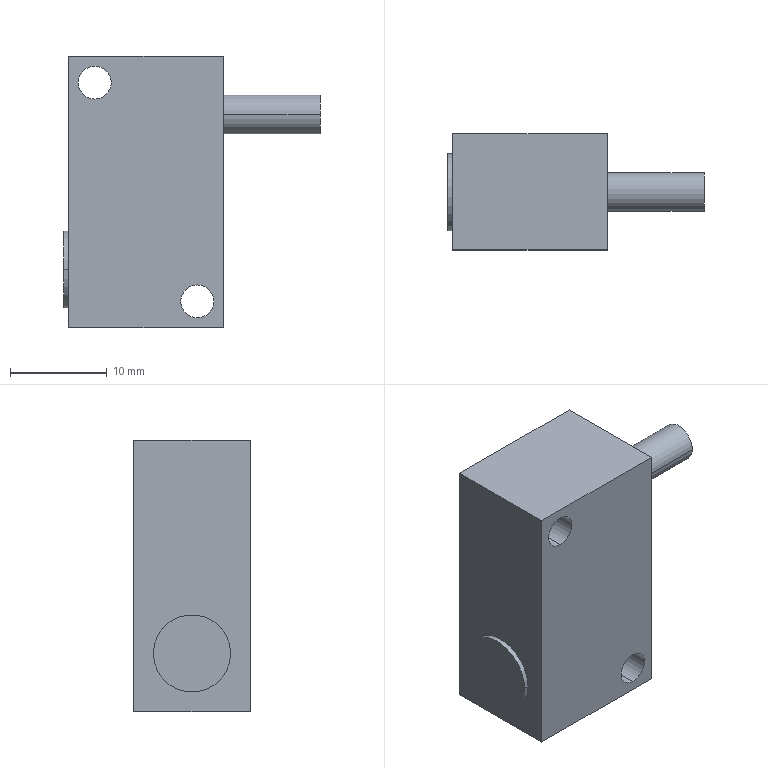Part | STEP file | Square proximity switch | 1 solid | 16 faces | box 26.5 x 12 x 28 mm | volume 5309 mm3 | cylinder 8 | plane 8 | commonest cylinder face diameters 3.4 x4 4 x2 8 x2
STEP:
#1=CARTESIAN_POINT('',(0.,0.,0.));
#2=DIRECTION('',(0.,0.,1.));
#3=DIRECTION('',(1.,0.,0.));
#4=AXIS2_PLACEMENT_3D('',#1,#2,#3);
#5=CARTESIAN_POINT('',(-5.3,6.,23.6));
#6=VERTEX_POINT('',#5);
#7=CARTESIAN_POINT('',(-5.3,-6.,23.6));
#8=VERTEX_POINT('',#7);
#9=CARTESIAN_POINT('',(-5.3,-6.,23.6));
#10=DIRECTION('',(0.,-1.,0.));
#11=VECTOR('',#10,1.);
#12=LINE('',#9,#11);
#13=CARTESIAN_POINT('',(-5.3,-6.,25.3));
#14=DIRECTION('',(0.,-1.,0.));
#15=DIRECTION('',(0.,0.,-1.));
#16=AXIS2_PLACEMENT_3D('',#13,#14,#15);
#17=CYLINDRICAL_SURFACE('',#16,1.7);
#18=CARTESIAN_POINT('',(6.283,0.));
#19=DIRECTION('',(0.,1.));
#20=VECTOR('',#19,1.);
#21=LINE('',#18,#20);
#22=(GEOMETRIC_REPRESENTATION_CONTEXT(2)PARAMETRIC_REPRESENTATION_CONTEXT()REPRESENTATION_CONTEXT('',''));
#23=DEFINITIONAL_REPRESENTATION('',(#21),#22);
#24=PCURVE('',#17,#23);
#25=CARTESIAN_POINT('',(-5.3,-6.,25.3));
#26=DIRECTION('',(0.,-1.,0.));
#27=DIRECTION('',(0.,0.,-1.));
#28=AXIS2_PLACEMENT_3D('',#25,#26,#27);
#29=CYLINDRICAL_SURFACE('',#28,1.7);
#30=CARTESIAN_POINT('',(0.,0.));
#31=DIRECTION('',(0.,1.));
#32=VECTOR('',#31,1.);
#33=LINE('',#30,#32);
#34=(GEOMETRIC_REPRESENTATION_CONTEXT(2)PARAMETRIC_REPRESENTATION_CONTEXT()REPRESENTATION_CONTEXT('',''));
#35=DEFINITIONAL_REPRESENTATION('',(#33),#34);
#36=PCURVE('',#29,#35);
#37=SURFACE_CURVE('',#12,(#24,#36),.PCURVE_S1.);
#38=EDGE_CURVE('',#6,#8,#37,.T.);
#39=ORIENTED_EDGE('',*,*,#38,.T.);
#40=CARTESIAN_POINT('',(-5.3,-6.,27.));
#41=VERTEX_POINT('',#40);
#42=CARTESIAN_POINT('',(-5.3,-6.,25.3));
#43=DIRECTION('',(0.,-1.,0.));
#44=DIRECTION('',(0.,0.,-1.));
#45=AXIS2_PLACEMENT_3D('',#42,#43,#44);
#46=CIRCLE('',#45,1.7);
#47=CARTESIAN_POINT('',(0.,0.));
#48=DIRECTION('',(1.,0.));
#49=VECTOR('',#48,1.);
#50=LINE('',#47,#49);
#51=(GEOMETRIC_REPRESENTATION_CONTEXT(2)PARAMETRIC_REPRESENTATION_CONTEXT()REPRESENTATION_CONTEXT('',''));
#52=DEFINITIONAL_REPRESENTATION('',(#50),#51);
#53=PCURVE('',#17,#52);
#54=CARTESIAN_POINT('',(-8.,-6.,28.));
#55=DIRECTION('',(0.,1.,0.));
#56=DIRECTION('',(0.,0.,1.));
#57=AXIS2_PLACEMENT_3D('',#54,#55,#56);
#58=PLANE('',#57);
#59=CARTESIAN_POINT('',(-4.4,2.7));
#60=CARTESIAN_POINT('',(-4.4,5.644));
#61=CARTESIAN_POINT('',(-1.85,4.172));
#62=CARTESIAN_POINT('',(0.7,2.7));
#63=CARTESIAN_POINT('',(-1.85,1.228));
#64=CARTESIAN_POINT('',(-4.4,-0.2445));
#65=CARTESIAN_POINT('',(-4.4,2.7));
#66=(BOUNDED_CURVE()B_SPLINE_CURVE(2,(#59,#60,#61,#62,#63,#64,#65),.UNSPECIFIED.,.T.,.F.)B_SPLINE_CURVE_WITH_KNOTS((1,2,2,2,2,1),(-2.094,0.,2.094,4.189,6.283,8.378),.UNSPECIFIED.)CURVE()GEOMETRIC_REPRESENTATION_ITEM()RATIONAL_B_SPLINE_CURVE((1.,0.5,1.,0.5,1.,0.5,1.))REPRESENTATION_ITEM(''));
#67=(GEOMETRIC_REPRESENTATION_CONTEXT(2)PARAMETRIC_REPRESENTATION_CONTEXT()REPRESENTATION_CONTEXT('',''));
#68=DEFINITIONAL_REPRESENTATION('',(#66),#67);
#69=PCURVE('',#58,#68);
#70=SURFACE_CURVE('',#46,(#53,#69),.PCURVE_S1.);
#71=EDGE_CURVE('',#41,#8,#70,.T.);
#72=ORIENTED_EDGE('',*,*,#71,.F.);
#73=CARTESIAN_POINT('',(-5.3,6.,27.));
#74=VERTEX_POINT('',#73);
#75=CARTESIAN_POINT('',(-5.3,-6.,27.));
#76=DIRECTION('',(0.,-1.,0.));
#77=VECTOR('',#76,1.);
#78=LINE('',#75,#77);
#79=CARTESIAN_POINT('',(3.142,0.));
#80=DIRECTION('',(0.,1.));
#81=VECTOR('',#80,1.);
#82=LINE('',#79,#81);
#83=(GEOMETRIC_REPRESENTATION_CONTEXT(2)PARAMETRIC_REPRESENTATION_CONTEXT()REPRESENTATION_CONTEXT('',''));
#84=DEFINITIONAL_REPRESENTATION('',(#82),#83);
#85=PCURVE('',#17,#84);
#86=CARTESIAN_POINT('',(3.142,0.));
#87=DIRECTION('',(0.,1.));
#88=VECTOR('',#87,1.);
#89=LINE('',#86,#88);
#90=(GEOMETRIC_REPRESENTATION_CONTEXT(2)PARAMETRIC_REPRESENTATION_CONTEXT()REPRESENTATION_CONTEXT('',''));
#91=DEFINITIONAL_REPRESENTATION('',(#89),#90);
#92=PCURVE('',#29,#91);
#93=SURFACE_CURVE('',#78,(#85,#92),.PCURVE_S1.);
#94=EDGE_CURVE('',#74,#41,#93,.T.);
#95=ORIENTED_EDGE('',*,*,#94,.F.);
#96=CARTESIAN_POINT('',(-5.3,6.,25.3));
#97=DIRECTION('',(0.,-1.,0.));
#98=DIRECTION('',(0.,0.,-1.));
#99=AXIS2_PLACEMENT_3D('',#96,#97,#98);
#100=CIRCLE('',#99,1.7);
#101=CARTESIAN_POINT('',(0.,-12.));
#102=DIRECTION('',(1.,0.));
#103=VECTOR('',#102,1.);
#104=LINE('',#101,#103);
#105=(GEOMETRIC_REPRESENTATION_CONTEXT(2)PARAMETRIC_REPRESENTATION_CONTEXT()REPRESENTATION_CONTEXT('',''));
#106=DEFINITIONAL_REPRESENTATION('',(#104),#105);
#107=PCURVE('',#17,#106);
#108=CARTESIAN_POINT('',(-8.,6.,28.));
#109=DIRECTION('',(0.,-1.,0.));
#110=DIRECTION('',(0.,0.,-1.));
#111=AXIS2_PLACEMENT_3D('',#108,#109,#110);
#112=PLANE('',#111);
#113=CARTESIAN_POINT('',(2.7,2.7));
#114=DIRECTION('',(1.,0.));
#115=AXIS2_PLACEMENT_2D('',#113,#114);
#116=CIRCLE('',#115,1.7);
#117=(GEOMETRIC_REPRESENTATION_CONTEXT(2)PARAMETRIC_REPRESENTATION_CONTEXT()REPRESENTATION_CONTEXT('',''));
#118=DEFINITIONAL_REPRESENTATION('',(#116),#117);
#119=PCURVE('',#112,#118);
#120=SURFACE_CURVE('',#100,(#107,#119),.PCURVE_S1.);
#121=EDGE_CURVE('',#74,#6,#120,.T.);
#122=ORIENTED_EDGE('',*,*,#121,.T.);
#123=EDGE_LOOP('',(#39,#72,#95,#122));
#124=FACE_BOUND('',#123,.F.);
#125=ADVANCED_FACE('',(#124),#17,.F.);
#126=CARTESIAN_POINT('',(5.3,6.,1.));
#127=VERTEX_POINT('',#126);
#128=CARTESIAN_POINT('',(5.3,-6.,1.));
#129=VERTEX_POINT('',#128);
#130=CARTESIAN_POINT('',(5.3,-6.,1.));
#131=DIRECTION('',(0.,-1.,0.));
#132=VECTOR('',#131,1.);
#133=LINE('',#130,#132);
#134=CARTESIAN_POINT('',(5.3,-6.,2.7));
#135=DIRECTION('',(0.,-1.,0.));
#136=DIRECTION('',(0.,0.,-1.));
#137=AXIS2_PLACEMENT_3D('',#134,#135,#136);
#138=CYLINDRICAL_SURFACE('',#137,1.7);
#139=CARTESIAN_POINT('',(6.283,0.));
#140=DIRECTION('',(0.,1.));
#141=VECTOR('',#140,1.);
#142=LINE('',#139,#141);
#143=(GEOMETRIC_REPRESENTATION_CONTEXT(2)PARAMETRIC_REPRESENTATION_CONTEXT()REPRESENTATION_CONTEXT('',''));
#144=DEFINITIONAL_REPRESENTATION('',(#142),#143);
#145=PCURVE('',#138,#144);
#146=CARTESIAN_POINT('',(5.3,-6.,2.7));
#147=DIRECTION('',(0.,-1.,0.));
#148=DIRECTION('',(0.,0.,-1.));
#149=AXIS2_PLACEMENT_3D('',#146,#147,#148);
#150=CYLINDRICAL_SURFACE('',#149,1.7);
#151=CARTESIAN_POINT('',(0.,0.));
#152=DIRECTION('',(0.,1.));
#153=VECTOR('',#152,1.);
#154=LINE('',#151,#153);
#155=(GEOMETRIC_REPRESENTATION_CONTEXT(2)PARAMETRIC_REPRESENTATION_CONTEXT()REPRESENTATION_CONTEXT('',''));
#156=DEFINITIONAL_REPRESENTATION('',(#154),#155);
#157=PCURVE('',#150,#156);
#158=SURFACE_CURVE('',#133,(#145,#157),.PCURVE_S1.);
#159=EDGE_CURVE('',#127,#129,#158,.T.);
#160=ORIENTED_EDGE('',*,*,#159,.T.);
#161=CARTESIAN_POINT('',(5.3,-6.,4.4));
#162=VERTEX_POINT('',#161);
#163=CARTESIAN_POINT('',(5.3,-6.,2.7));
#164=DIRECTION('',(0.,-1.,0.));
#165=DIRECTION('',(0.,0.,-1.));
#166=AXIS2_PLACEMENT_3D('',#163,#164,#165);
#167=CIRCLE('',#166,1.7);
#168=CARTESIAN_POINT('',(0.,0.));
#169=DIRECTION('',(1.,0.));
#170=VECTOR('',#169,1.);
#171=LINE('',#168,#170);
#172=(GEOMETRIC_REPRESENTATION_CONTEXT(2)PARAMETRIC_REPRESENTATION_CONTEXT()REPRESENTATION_CONTEXT('',''));
#173=DEFINITIONAL_REPRESENTATION('',(#171),#172);
#174=PCURVE('',#138,#173);
#175=CARTESIAN_POINT('',(-27.,13.3));
#176=CARTESIAN_POINT('',(-27.,16.244));
#177=CARTESIAN_POINT('',(-24.45,14.772));
#178=CARTESIAN_POINT('',(-21.9,13.3));
#179=CARTESIAN_POINT('',(-24.45,11.828));
#180=CARTESIAN_POINT('',(-27.,10.356));
#181=CARTESIAN_POINT('',(-27.,13.3));
#182=(BOUNDED_CURVE()B_SPLINE_CURVE(2,(#175,#176,#177,#178,#179,#180,#181),.UNSPECIFIED.,.T.,.F.)B_SPLINE_CURVE_WITH_KNOTS((1,2,2,2,2,1),(-2.094,0.,2.094,4.189,6.283,8.378),.UNSPECIFIED.)CURVE()GEOMETRIC_REPRESENTATION_ITEM()RATIONAL_B_SPLINE_CURVE((1.,0.5,1.,0.5,1.,0.5,1.))REPRESENTATION_ITEM(''));
#183=(GEOMETRIC_REPRESENTATION_CONTEXT(2)PARAMETRIC_REPRESENTATION_CONTEXT()REPRESENTATION_CONTEXT('',''));
#184=DEFINITIONAL_REPRESENTATION('',(#182),#183);
#185=PCURVE('',#58,#184);
#186=SURFACE_CURVE('',#167,(#174,#185),.PCURVE_S1.);
#187=EDGE_CURVE('',#162,#129,#186,.T.);
#188=ORIENTED_EDGE('',*,*,#187,.F.);
#189=CARTESIAN_POINT('',(5.3,6.,4.4));
#190=VERTEX_POINT('',#189);
#191=CARTESIAN_POINT('',(5.3,-6.,4.4));
#192=DIRECTION('',(0.,-1.,0.));
#193=VECTOR('',#192,1.);
#194=LINE('',#191,#193);
#195=CARTESIAN_POINT('',(3.142,0.));
#196=DIRECTION('',(0.,1.));
#197=VECTOR('',#196,1.);
#198=LINE('',#195,#197);
#199=(GEOMETRIC_REPRESENTATION_CONTEXT(2)PARAMETRIC_REPRESENTATION_CONTEXT()REPRESENTATION_CONTEXT('',''));
#200=DEFINITIONAL_REPRESENTATION('',(#198),#199);
#201=PCURVE('',#138,#200);
#202=CARTESIAN_POINT('',(3.142,0.));
#203=DIRECTION('',(0.,1.));
#204=VECTOR('',#203,1.);
#205=LINE('',#202,#204);
#206=(GEOMETRIC_REPRESENTATION_CONTEXT(2)PARAMETRIC_REPRESENTATION_CONTEXT()REPRESENTATION_CONTEXT('',''));
#207=DEFINITIONAL_REPRESENTATION('',(#205),#206);
#208=PCURVE('',#150,#207);
#209=SURFACE_CURVE('',#194,(#201,#208),.PCURVE_S1.);
#210=EDGE_CURVE('',#190,#162,#209,.T.);
#211=ORIENTED_EDGE('',*,*,#210,.F.);
#212=CARTESIAN_POINT('',(5.3,6.,2.7));
#213=DIRECTION('',(0.,-1.,0.));
#214=DIRECTION('',(0.,0.,-1.));
#215=AXIS2_PLACEMENT_3D('',#212,#213,#214);
#216=CIRCLE('',#215,1.7);
#217=CARTESIAN_POINT('',(0.,-12.));
#218=DIRECTION('',(1.,0.));
#219=VECTOR('',#218,1.);
#220=LINE('',#217,#219);
#221=(GEOMETRIC_REPRESENTATION_CONTEXT(2)PARAMETRIC_REPRESENTATION_CONTEXT()REPRESENTATION_CONTEXT('',''));
#222=DEFINITIONAL_REPRESENTATION('',(#220),#221);
#223=PCURVE('',#138,#222);
#224=CARTESIAN_POINT('',(25.3,13.3));
#225=DIRECTION('',(1.,0.));
#226=AXIS2_PLACEMENT_2D('',#224,#225);
#227=CIRCLE('',#226,1.7);
#228=(GEOMETRIC_REPRESENTATION_CONTEXT(2)PARAMETRIC_REPRESENTATION_CONTEXT()REPRESENTATION_CONTEXT('',''));
#229=DEFINITIONAL_REPRESENTATION('',(#227),#228);
#230=PCURVE('',#112,#229);
#231=SURFACE_CURVE('',#216,(#223,#230),.PCURVE_S1.);
#232=EDGE_CURVE('',#190,#127,#231,.T.);
#233=ORIENTED_EDGE('',*,*,#232,.T.);
#234=EDGE_LOOP('',(#160,#188,#211,#233));
#235=FACE_BOUND('',#234,.F.);
#236=ADVANCED_FACE('',(#235),#138,.F.);
#237=CARTESIAN_POINT('',(18.,2.,22.));
#238=VERTEX_POINT('',#237);
#239=CARTESIAN_POINT('',(18.,-2.,22.));
#240=VERTEX_POINT('',#239);
#241=CARTESIAN_POINT('',(18.,0.,22.));
#242=DIRECTION('',(1.,0.,0.));
#243=DIRECTION('',(0.,1.,0.));
#244=AXIS2_PLACEMENT_3D('',#241,#242,#243);
#245=CIRCLE('',#244,2.);
#246=CARTESIAN_POINT('',(18.,0.,22.));
#247=DIRECTION('',(-1.,0.,0.));
#248=DIRECTION('',(0.,-1.,0.));
#249=AXIS2_PLACEMENT_3D('',#246,#247,#248);
#250=CYLINDRICAL_SURFACE('',#249,2.);
#251=CARTESIAN_POINT('',(3.142,0.));
#252=DIRECTION('',(-1.,0.));
#253=VECTOR('',#252,1.);
#254=LINE('',#251,#253);
#255=(GEOMETRIC_REPRESENTATION_CONTEXT(2)PARAMETRIC_REPRESENTATION_CONTEXT()REPRESENTATION_CONTEXT('',''));
#256=DEFINITIONAL_REPRESENTATION('',(#254),#255);
#257=PCURVE('',#250,#256);
#258=CARTESIAN_POINT('',(18.,0.,22.));
#259=DIRECTION('',(1.,0.,0.));
#260=DIRECTION('',(0.,1.,0.));
#261=AXIS2_PLACEMENT_3D('',#258,#259,#260);
#262=PLANE('',#261);
#263=CARTESIAN_POINT('',(0.,0.));
#264=DIRECTION('',(1.,0.));
#265=AXIS2_PLACEMENT_2D('',#263,#264);
#266=CIRCLE('',#265,2.);
#267=(GEOMETRIC_REPRESENTATION_CONTEXT(2)PARAMETRIC_REPRESENTATION_CONTEXT()REPRESENTATION_CONTEXT('',''));
#268=DEFINITIONAL_REPRESENTATION('',(#266),#267);
#269=PCURVE('',#262,#268);
#270=SURFACE_CURVE('',#245,(#257,#269),.PCURVE_S1.);
#271=EDGE_CURVE('',#238,#240,#270,.T.);
#272=ORIENTED_EDGE('',*,*,#271,.F.);
#273=CARTESIAN_POINT('',(8.,2.,22.));
#274=VERTEX_POINT('',#273);
#275=CARTESIAN_POINT('',(18.,2.,22.));
#276=DIRECTION('',(-1.,0.,0.));
#277=VECTOR('',#276,1.);
#278=LINE('',#275,#277);
#279=CARTESIAN_POINT('',(3.142,0.));
#280=DIRECTION('',(0.,1.));
#281=VECTOR('',#280,1.);
#282=LINE('',#279,#281);
#283=(GEOMETRIC_REPRESENTATION_CONTEXT(2)PARAMETRIC_REPRESENTATION_CONTEXT()REPRESENTATION_CONTEXT('',''));
#284=DEFINITIONAL_REPRESENTATION('',(#282),#283);
#285=PCURVE('',#250,#284);
#286=CARTESIAN_POINT('',(18.,0.,22.));
#287=DIRECTION('',(-1.,0.,0.));
#288=DIRECTION('',(0.,-1.,0.));
#289=AXIS2_PLACEMENT_3D('',#286,#287,#288);
#290=CYLINDRICAL_SURFACE('',#289,2.);
#291=CARTESIAN_POINT('',(3.142,0.));
#292=DIRECTION('',(0.,1.));
#293=VECTOR('',#292,1.);
#294=LINE('',#291,#293);
#295=(GEOMETRIC_REPRESENTATION_CONTEXT(2)PARAMETRIC_REPRESENTATION_CONTEXT()REPRESENTATION_CONTEXT('',''));
#296=DEFINITIONAL_REPRESENTATION('',(#294),#295);
#297=PCURVE('',#290,#296);
#298=SURFACE_CURVE('',#278,(#285,#297),.PCURVE_S1.);
#299=EDGE_CURVE('',#238,#274,#298,.T.);
#300=ORIENTED_EDGE('',*,*,#299,.T.);
#301=CARTESIAN_POINT('',(8.,-2.,22.));
#302=VERTEX_POINT('',#301);
#303=CARTESIAN_POINT('',(8.,0.,22.));
#304=DIRECTION('',(1.,0.,0.));
#305=DIRECTION('',(0.,-1.,0.));
#306=AXIS2_PLACEMENT_3D('',#303,#304,#305);
#307=CIRCLE('',#306,2.);
#308=CARTESIAN_POINT('',(6.283,10.));
#309=DIRECTION('',(-1.,0.));
#310=VECTOR('',#309,1.);
#311=LINE('',#308,#310);
#312=(GEOMETRIC_REPRESENTATION_CONTEXT(2)PARAMETRIC_REPRESENTATION_CONTEXT()REPRESENTATION_CONTEXT('',''));
#313=DEFINITIONAL_REPRESENTATION('',(#311),#312);
#314=PCURVE('',#250,#313);
#315=CARTESIAN_POINT('',(8.,6.,28.));
#316=DIRECTION('',(-1.,0.,0.));
#317=DIRECTION('',(0.,-1.,0.));
#318=AXIS2_PLACEMENT_3D('',#315,#316,#317);
#319=PLANE('',#318);
#320=CARTESIAN_POINT('',(8.,-6.));
#321=CARTESIAN_POINT('',(8.,-9.464));
#322=CARTESIAN_POINT('',(5.,-7.732));
#323=CARTESIAN_POINT('',(2.,-6.));
#324=CARTESIAN_POINT('',(5.,-4.268));
#325=CARTESIAN_POINT('',(8.,-2.536));
#326=CARTESIAN_POINT('',(8.,-6.));
#327=(BOUNDED_CURVE()B_SPLINE_CURVE(2,(#320,#321,#322,#323,#324,#325,#326),.UNSPECIFIED.,.T.,.F.)B_SPLINE_CURVE_WITH_KNOTS((1,2,2,2,2,1),(-2.094,0.,2.094,4.189,6.283,8.378),.UNSPECIFIED.)CURVE()GEOMETRIC_REPRESENTATION_ITEM()RATIONAL_B_SPLINE_CURVE((1.,0.5,1.,0.5,1.,0.5,1.))REPRESENTATION_ITEM(''));
#328=(GEOMETRIC_REPRESENTATION_CONTEXT(2)PARAMETRIC_REPRESENTATION_CONTEXT()REPRESENTATION_CONTEXT('',''));
#329=DEFINITIONAL_REPRESENTATION('',(#327),#328);
#330=PCURVE('',#319,#329);
#331=SURFACE_CURVE('',#307,(#314,#330),.PCURVE_S1.);
#332=EDGE_CURVE('',#274,#302,#331,.T.);
#333=ORIENTED_EDGE('',*,*,#332,.T.);
#334=CARTESIAN_POINT('',(18.,-2.,22.));
#335=DIRECTION('',(-1.,0.,0.));
#336=VECTOR('',#335,1.);
#337=LINE('',#334,#336);
#338=CARTESIAN_POINT('',(0.,0.));
#339=DIRECTION('',(0.,1.));
#340=VECTOR('',#339,1.);
#341=LINE('',#338,#340);
#342=(GEOMETRIC_REPRESENTATION_CONTEXT(2)PARAMETRIC_REPRESENTATION_CONTEXT()REPRESENTATION_CONTEXT('',''));
#343=DEFINITIONAL_REPRESENTATION('',(#341),#342);
#344=PCURVE('',#250,#343);
#345=CARTESIAN_POINT('',(6.283,0.));
#346=DIRECTION('',(0.,1.));
#347=VECTOR('',#346,1.);
#348=LINE('',#345,#347);
#349=(GEOMETRIC_REPRESENTATION_CONTEXT(2)PARAMETRIC_REPRESENTATION_CONTEXT()REPRESENTATION_CONTEXT('',''));
#350=DEFINITIONAL_REPRESENTATION('',(#348),#349);
#351=PCURVE('',#290,#350);
#352=SURFACE_CURVE('',#337,(#344,#351),.PCURVE_S1.);
#353=EDGE_CURVE('',#240,#302,#352,.T.);
#354=ORIENTED_EDGE('',*,*,#353,.F.);
#355=EDGE_LOOP('',(#272,#300,#333,#354));
#356=FACE_BOUND('',#355,.T.);
#357=ADVANCED_FACE('',(#356),#250,.T.);
#358=CARTESIAN_POINT('',(-8.5,-4.,6.));
#359=VERTEX_POINT('',#358);
#360=CARTESIAN_POINT('',(-8.5,4.,6.));
#361=VERTEX_POINT('',#360);
#362=CARTESIAN_POINT('',(-8.5,0.,6.));
#363=DIRECTION('',(-1.,0.,0.));
#364=DIRECTION('',(0.,-1.,0.));
#365=AXIS2_PLACEMENT_3D('',#362,#363,#364);
#366=CIRCLE('',#365,4.);
#367=CARTESIAN_POINT('',(-8.5,0.,6.));
#368=DIRECTION('',(1.,0.,0.));
#369=DIRECTION('',(0.,1.,0.));
#370=AXIS2_PLACEMENT_3D('',#367,#368,#369);
#371=CYLINDRICAL_SURFACE('',#370,4.);
#372=CARTESIAN_POINT('',(3.142,0.));
#373=DIRECTION('',(-1.,0.));
#374=VECTOR('',#373,1.);
#375=LINE('',#372,#374);
#376=(GEOMETRIC_REPRESENTATION_CONTEXT(2)PARAMETRIC_REPRESENTATION_CONTEXT()REPRESENTATION_CONTEXT('',''));
#377=DEFINITIONAL_REPRESENTATION('',(#375),#376);
#378=PCURVE('',#371,#377);
#379=CARTESIAN_POINT('',(-8.5,0.,6.));
#380=DIRECTION('',(-1.,0.,0.));
#381=DIRECTION('',(0.,-1.,0.));
#382=AXIS2_PLACEMENT_3D('',#379,#380,#381);
#383=PLANE('',#382);
#384=CARTESIAN_POINT('',(0.,0.));
#385=DIRECTION('',(1.,0.));
#386=AXIS2_PLACEMENT_2D('',#384,#385);
#387=CIRCLE('',#386,4.);
#388=(GEOMETRIC_REPRESENTATION_CONTEXT(2)PARAMETRIC_REPRESENTATION_CONTEXT()REPRESENTATION_CONTEXT('',''));
#389=DEFINITIONAL_REPRESENTATION('',(#387),#388);
#390=PCURVE('',#383,#389);
#391=SURFACE_CURVE('',#366,(#378,#390),.PCURVE_S1.);
#392=EDGE_CURVE('',#359,#361,#391,.T.);
#393=ORIENTED_EDGE('',*,*,#392,.F.);
#394=CARTESIAN_POINT('',(-8.,-4.,6.));
#395=VERTEX_POINT('',#394);
#396=CARTESIAN_POINT('',(-8.5,-4.,6.));
#397=DIRECTION('',(1.,0.,0.));
#398=VECTOR('',#397,1.);
#399=LINE('',#396,#398);
#400=CARTESIAN_POINT('',(3.142,0.));
#401=DIRECTION('',(0.,1.));
#402=VECTOR('',#401,1.);
#403=LINE('',#400,#402);
#404=(GEOMETRIC_REPRESENTATION_CONTEXT(2)PARAMETRIC_REPRESENTATION_CONTEXT()REPRESENTATION_CONTEXT('',''));
#405=DEFINITIONAL_REPRESENTATION('',(#403),#404);
#406=PCURVE('',#371,#405);
#407=CARTESIAN_POINT('',(-8.5,0.,6.));
#408=DIRECTION('',(1.,0.,0.));
#409=DIRECTION('',(0.,1.,0.));
#410=AXIS2_PLACEMENT_3D('',#407,#408,#409);
#411=CYLINDRICAL_SURFACE('',#410,4.);
#412=CARTESIAN_POINT('',(3.142,0.));
#413=DIRECTION('',(0.,1.));
#414=VECTOR('',#413,1.);
#415=LINE('',#412,#414);
#416=(GEOMETRIC_REPRESENTATION_CONTEXT(2)PARAMETRIC_REPRESENTATION_CONTEXT()REPRESENTATION_CONTEXT('',''));
#417=DEFINITIONAL_REPRESENTATION('',(#415),#416);
#418=PCURVE('',#411,#417);
#419=SURFACE_CURVE('',#399,(#406,#418),.PCURVE_S1.);
#420=EDGE_CURVE('',#359,#395,#419,.T.);
#421=ORIENTED_EDGE('',*,*,#420,.T.);
#422=CARTESIAN_POINT('',(-8.,4.,6.));
#423=VERTEX_POINT('',#422);
#424=CARTESIAN_POINT('',(-8.,0.,6.));
#425=DIRECTION('',(-1.,0.,0.));
#426=DIRECTION('',(0.,1.,0.));
#427=AXIS2_PLACEMENT_3D('',#424,#425,#426);
#428=CIRCLE('',#427,4.);
#429=CARTESIAN_POINT('',(6.283,0.5));
#430=DIRECTION('',(-1.,0.));
#431=VECTOR('',#430,1.);
#432=LINE('',#429,#431);
#433=(GEOMETRIC_REPRESENTATION_CONTEXT(2)PARAMETRIC_REPRESENTATION_CONTEXT()REPRESENTATION_CONTEXT('',''));
#434=DEFINITIONAL_REPRESENTATION('',(#432),#433);
#435=PCURVE('',#371,#434);
#436=CARTESIAN_POINT('',(-8.,6.,28.));
#437=DIRECTION('',(1.,0.,0.));
#438=DIRECTION('',(0.,1.,0.));
#439=AXIS2_PLACEMENT_3D('',#436,#437,#438);
#440=PLANE('',#439);
#441=CARTESIAN_POINT('',(-2.,-22.));
#442=CARTESIAN_POINT('',(-2.,-28.928));
#443=CARTESIAN_POINT('',(-8.,-25.464));
#444=CARTESIAN_POINT('',(-14.,-22.));
#445=CARTESIAN_POINT('',(-8.,-18.536));
#446=CARTESIAN_POINT('',(-2.,-15.072));
#447=CARTESIAN_POINT('',(-2.,-22.));
#448=(BOUNDED_CURVE()B_SPLINE_CURVE(2,(#441,#442,#443,#444,#445,#446,#447),.UNSPECIFIED.,.T.,.F.)B_SPLINE_CURVE_WITH_KNOTS((1,2,2,2,2,1),(-2.094,0.,2.094,4.189,6.283,8.378),.UNSPECIFIED.)CURVE()GEOMETRIC_REPRESENTATION_ITEM()RATIONAL_B_SPLINE_CURVE((1.,0.5,1.,0.5,1.,0.5,1.))REPRESENTATION_ITEM(''));
#449=(GEOMETRIC_REPRESENTATION_CONTEXT(2)PARAMETRIC_REPRESENTATION_CONTEXT()REPRESENTATION_CONTEXT('',''));
#450=DEFINITIONAL_REPRESENTATION('',(#448),#449);
#451=PCURVE('',#440,#450);
#452=SURFACE_CURVE('',#428,(#435,#451),.PCURVE_S1.);
#453=EDGE_CURVE('',#395,#423,#452,.T.);
#454=ORIENTED_EDGE('',*,*,#453,.T.);
#455=CARTESIAN_POINT('',(-8.5,4.,6.));
#456=DIRECTION('',(1.,0.,0.));
#457=VECTOR('',#456,1.);
#458=LINE('',#455,#457);
#459=CARTESIAN_POINT('',(0.,0.));
#460=DIRECTION('',(0.,1.));
#461=VECTOR('',#460,1.);
#462=LINE('',#459,#461);
#463=(GEOMETRIC_REPRESENTATION_CONTEXT(2)PARAMETRIC_REPRESENTATION_CONTEXT()REPRESENTATION_CONTEXT('',''));
#464=DEFINITIONAL_REPRESENTATION('',(#462),#463);
#465=PCURVE('',#371,#464);
#466=CARTESIAN_POINT('',(6.283,0.));
#467=DIRECTION('',(0.,1.));
#468=VECTOR('',#467,1.);
#469=LINE('',#466,#468);
#470=(GEOMETRIC_REPRESENTATION_CONTEXT(2)PARAMETRIC_REPRESENTATION_CONTEXT()REPRESENTATION_CONTEXT('',''));
#471=DEFINITIONAL_REPRESENTATION('',(#469),#470);
#472=PCURVE('',#411,#471);
#473=SURFACE_CURVE('',#458,(#465,#472),.PCURVE_S1.);
#474=EDGE_CURVE('',#361,#423,#473,.T.);
#475=ORIENTED_EDGE('',*,*,#474,.F.);
#476=EDGE_LOOP('',(#393,#421,#454,#475));
#477=FACE_BOUND('',#476,.T.);
#478=ADVANCED_FACE('',(#477),#371,.T.);
#479=CARTESIAN_POINT('',(-5.3,-6.,25.3));
#480=DIRECTION('',(0.,-1.,0.));
#481=DIRECTION('',(0.,0.,-1.));
#482=AXIS2_PLACEMENT_3D('',#479,#480,#481);
#483=CIRCLE('',#482,1.7);
#484=CARTESIAN_POINT('',(-4.4,2.7));
#485=CARTESIAN_POINT('',(-4.4,5.644));
#486=CARTESIAN_POINT('',(-1.85,4.172));
#487=CARTESIAN_POINT('',(0.7,2.7));
#488=CARTESIAN_POINT('',(-1.85,1.228));
#489=CARTESIAN_POINT('',(-4.4,-0.2445));
#490=CARTESIAN_POINT('',(-4.4,2.7));
#491=(BOUNDED_CURVE()B_SPLINE_CURVE(2,(#484,#485,#486,#487,#488,#489,#490),.UNSPECIFIED.,.T.,.F.)B_SPLINE_CURVE_WITH_KNOTS((1,2,2,2,2,1),(-2.094,0.,2.094,4.189,6.283,8.378),.UNSPECIFIED.)CURVE()GEOMETRIC_REPRESENTATION_ITEM()RATIONAL_B_SPLINE_CURVE((1.,0.5,1.,0.5,1.,0.5,1.))REPRESENTATION_ITEM(''));
#492=(GEOMETRIC_REPRESENTATION_CONTEXT(2)PARAMETRIC_REPRESENTATION_CONTEXT()REPRESENTATION_CONTEXT('',''));
#493=DEFINITIONAL_REPRESENTATION('',(#491),#492);
#494=PCURVE('',#58,#493);
#495=CARTESIAN_POINT('',(0.,0.));
#496=DIRECTION('',(1.,0.));
#497=VECTOR('',#496,1.);
#498=LINE('',#495,#497);
#499=(GEOMETRIC_REPRESENTATION_CONTEXT(2)PARAMETRIC_REPRESENTATION_CONTEXT()REPRESENTATION_CONTEXT('',''));
#500=DEFINITIONAL_REPRESENTATION('',(#498),#499);
#501=PCURVE('',#29,#500);
#502=SURFACE_CURVE('',#483,(#494,#501),.PCURVE_S1.);
#503=EDGE_CURVE('',#8,#41,#502,.T.);
#504=ORIENTED_EDGE('',*,*,#503,.F.);
#505=ORIENTED_EDGE('',*,*,#71,.F.);
#506=EDGE_LOOP('',(#504,#505));
#507=FACE_BOUND('',#506,.T.);
#508=CARTESIAN_POINT('',(-8.,-6.,0.));
#509=VERTEX_POINT('',#508);
#510=CARTESIAN_POINT('',(8.,-6.,0.));
#511=VERTEX_POINT('',#510);
#512=CARTESIAN_POINT('',(-8.,-6.,0.));
#513=DIRECTION('',(1.,0.,0.));
#514=VECTOR('',#513,1.);
#515=LINE('',#512,#514);
#516=CARTESIAN_POINT('',(-28.,0.));
#517=DIRECTION('',(0.,1.));
#518=VECTOR('',#517,1.);
#519=LINE('',#516,#518);
#520=(GEOMETRIC_REPRESENTATION_CONTEXT(2)PARAMETRIC_REPRESENTATION_CONTEXT()REPRESENTATION_CONTEXT('',''));
#521=DEFINITIONAL_REPRESENTATION('',(#519),#520);
#522=PCURVE('',#58,#521);
#523=CARTESIAN_POINT('',(0.,0.,0.));
#524=DIRECTION('',(0.,0.,1.));
#525=DIRECTION('',(1.,0.,0.));
#526=AXIS2_PLACEMENT_3D('',#523,#524,#525);
#527=PLANE('',#526);
#528=CARTESIAN_POINT('',(-8.,-6.));
#529=DIRECTION('',(1.,0.));
#530=VECTOR('',#529,1.);
#531=LINE('',#528,#530);
#532=(GEOMETRIC_REPRESENTATION_CONTEXT(2)PARAMETRIC_REPRESENTATION_CONTEXT()REPRESENTATION_CONTEXT('',''));
#533=DEFINITIONAL_REPRESENTATION('',(#531),#532);
#534=PCURVE('',#527,#533);
#535=SURFACE_CURVE('',#515,(#522,#534),.PCURVE_S1.);
#536=EDGE_CURVE('',#509,#511,#535,.T.);
#537=ORIENTED_EDGE('',*,*,#536,.T.);
#538=CARTESIAN_POINT('',(8.,-6.,28.));
#539=VERTEX_POINT('',#538);
#540=CARTESIAN_POINT('',(8.,-6.,28.));
#541=DIRECTION('',(0.,0.,-1.));
#542=VECTOR('',#541,1.);
#543=LINE('',#540,#542);
#544=CARTESIAN_POINT('',(0.,16.));
#545=DIRECTION('',(-1.,0.));
#546=VECTOR('',#545,1.);
#547=LINE('',#544,#546);
#548=(GEOMETRIC_REPRESENTATION_CONTEXT(2)PARAMETRIC_REPRESENTATION_CONTEXT()REPRESENTATION_CONTEXT('',''));
#549=DEFINITIONAL_REPRESENTATION('',(#547),#548);
#550=PCURVE('',#58,#549);
#551=CARTESIAN_POINT('',(12.,0.));
#552=DIRECTION('',(0.,-1.));
#553=VECTOR('',#552,1.);
#554=LINE('',#551,#553);
#555=(GEOMETRIC_REPRESENTATION_CONTEXT(2)PARAMETRIC_REPRESENTATION_CONTEXT()REPRESENTATION_CONTEXT('',''));
#556=DEFINITIONAL_REPRESENTATION('',(#554),#555);
#557=PCURVE('',#319,#556);
#558=SURFACE_CURVE('',#543,(#550,#557),.PCURVE_S1.);
#559=EDGE_CURVE('',#539,#511,#558,.T.);
#560=ORIENTED_EDGE('',*,*,#559,.F.);
#561=CARTESIAN_POINT('',(-8.,-6.,28.));
#562=VERTEX_POINT('',#561);
#563=CARTESIAN_POINT('',(-8.,-6.,28.));
#564=DIRECTION('',(1.,0.,0.));
#565=VECTOR('',#564,1.);
#566=LINE('',#563,#565);
#567=CARTESIAN_POINT('',(0.,0.));
#568=DIRECTION('',(0.,1.));
#569=VECTOR('',#568,1.);
#570=LINE('',#567,#569);
#571=(GEOMETRIC_REPRESENTATION_CONTEXT(2)PARAMETRIC_REPRESENTATION_CONTEXT()REPRESENTATION_CONTEXT('',''));
#572=DEFINITIONAL_REPRESENTATION('',(#570),#571);
#573=PCURVE('',#58,#572);
#574=CARTESIAN_POINT('',(0.,0.,28.));
#575=DIRECTION('',(0.,0.,1.));
#576=DIRECTION('',(1.,0.,0.));
#577=AXIS2_PLACEMENT_3D('',#574,#575,#576);
#578=PLANE('',#577);
#579=CARTESIAN_POINT('',(-8.,-6.));
#580=DIRECTION('',(1.,0.));
#581=VECTOR('',#580,1.);
#582=LINE('',#579,#581);
#583=(GEOMETRIC_REPRESENTATION_CONTEXT(2)PARAMETRIC_REPRESENTATION_CONTEXT()REPRESENTATION_CONTEXT('',''));
#584=DEFINITIONAL_REPRESENTATION('',(#582),#583);
#585=PCURVE('',#578,#584);
#586=SURFACE_CURVE('',#566,(#573,#585),.PCURVE_S1.);
#587=EDGE_CURVE('',#562,#539,#586,.T.);
#588=ORIENTED_EDGE('',*,*,#587,.F.);
#589=CARTESIAN_POINT('',(-8.,-6.,28.));
#590=DIRECTION('',(0.,0.,-1.));
#591=VECTOR('',#590,1.);
#592=LINE('',#589,#591);
#593=CARTESIAN_POINT('',(0.,0.));
#594=DIRECTION('',(-1.,0.));
#595=VECTOR('',#594,1.);
#596=LINE('',#593,#595);
#597=(GEOMETRIC_REPRESENTATION_CONTEXT(2)PARAMETRIC_REPRESENTATION_CONTEXT()REPRESENTATION_CONTEXT('',''));
#598=DEFINITIONAL_REPRESENTATION('',(#596),#597);
#599=PCURVE('',#58,#598);
#600=CARTESIAN_POINT('',(-12.,0.));
#601=DIRECTION('',(0.,-1.));
#602=VECTOR('',#601,1.);
#603=LINE('',#600,#602);
#604=(GEOMETRIC_REPRESENTATION_CONTEXT(2)PARAMETRIC_REPRESENTATION_CONTEXT()REPRESENTATION_CONTEXT('',''));
#605=DEFINITIONAL_REPRESENTATION('',(#603),#604);
#606=PCURVE('',#440,#605);
#607=SURFACE_CURVE('',#592,(#599,#606),.PCURVE_S1.);
#608=EDGE_CURVE('',#562,#509,#607,.T.);
#609=ORIENTED_EDGE('',*,*,#608,.T.);
#610=EDGE_LOOP('',(#537,#560,#588,#609));
#611=FACE_BOUND('',#610,.T.);
#612=CARTESIAN_POINT('',(5.3,-6.,2.7));
#613=DIRECTION('',(0.,-1.,0.));
#614=DIRECTION('',(0.,0.,-1.));
#615=AXIS2_PLACEMENT_3D('',#612,#613,#614);
#616=CIRCLE('',#615,1.7);
#617=CARTESIAN_POINT('',(-27.,13.3));
#618=CARTESIAN_POINT('',(-27.,16.244));
#619=CARTESIAN_POINT('',(-24.45,14.772));
#620=CARTESIAN_POINT('',(-21.9,13.3));
#621=CARTESIAN_POINT('',(-24.45,11.828));
#622=CARTESIAN_POINT('',(-27.,10.356));
#623=CARTESIAN_POINT('',(-27.,13.3));
#624=(BOUNDED_CURVE()B_SPLINE_CURVE(2,(#617,#618,#619,#620,#621,#622,#623),.UNSPECIFIED.,.T.,.F.)B_SPLINE_CURVE_WITH_KNOTS((1,2,2,2,2,1),(-2.094,0.,2.094,4.189,6.283,8.378),.UNSPECIFIED.)CURVE()GEOMETRIC_REPRESENTATION_ITEM()RATIONAL_B_SPLINE_CURVE((1.,0.5,1.,0.5,1.,0.5,1.))REPRESENTATION_ITEM(''));
#625=(GEOMETRIC_REPRESENTATION_CONTEXT(2)PARAMETRIC_REPRESENTATION_CONTEXT()REPRESENTATION_CONTEXT('',''));
#626=DEFINITIONAL_REPRESENTATION('',(#624),#625);
#627=PCURVE('',#58,#626);
#628=CARTESIAN_POINT('',(0.,0.));
#629=DIRECTION('',(1.,0.));
#630=VECTOR('',#629,1.);
#631=LINE('',#628,#630);
#632=(GEOMETRIC_REPRESENTATION_CONTEXT(2)PARAMETRIC_REPRESENTATION_CONTEXT()REPRESENTATION_CONTEXT('',''));
#633=DEFINITIONAL_REPRESENTATION('',(#631),#632);
#634=PCURVE('',#150,#633);
#635=SURFACE_CURVE('',#616,(#627,#634),.PCURVE_S1.);
#636=EDGE_CURVE('',#129,#162,#635,.T.);
#637=ORIENTED_EDGE('',*,*,#636,.F.);
#638=ORIENTED_EDGE('',*,*,#187,.F.);
#639=EDGE_LOOP('',(#637,#638));
#640=FACE_BOUND('',#639,.T.);
#641=ADVANCED_FACE('',(#507,#611,#640),#58,.F.);
#642=CARTESIAN_POINT('',(8.,6.,0.));
#643=VERTEX_POINT('',#642);
#644=CARTESIAN_POINT('',(8.,6.,0.));
#645=DIRECTION('',(0.,1.,0.));
#646=VECTOR('',#645,1.);
#647=LINE('',#644,#646);
#648=CARTESIAN_POINT('',(0.,-28.));
#649=DIRECTION('',(-1.,0.));
#650=VECTOR('',#649,1.);
#651=LINE('',#648,#650);
#652=(GEOMETRIC_REPRESENTATION_CONTEXT(2)PARAMETRIC_REPRESENTATION_CONTEXT()REPRESENTATION_CONTEXT('',''));
#653=DEFINITIONAL_REPRESENTATION('',(#651),#652);
#654=PCURVE('',#319,#653);
#655=CARTESIAN_POINT('',(8.,6.));
#656=DIRECTION('',(0.,1.));
#657=VECTOR('',#656,1.);
#658=LINE('',#655,#657);
#659=(GEOMETRIC_REPRESENTATION_CONTEXT(2)PARAMETRIC_REPRESENTATION_CONTEXT()REPRESENTATION_CONTEXT('',''));
#660=DEFINITIONAL_REPRESENTATION('',(#658),#659);
#661=PCURVE('',#527,#660);
#662=SURFACE_CURVE('',#647,(#654,#661),.PCURVE_S1.);
#663=EDGE_CURVE('',#511,#643,#662,.T.);
#664=ORIENTED_EDGE('',*,*,#663,.T.);
#665=CARTESIAN_POINT('',(8.,6.,28.));
#666=VERTEX_POINT('',#665);
#667=CARTESIAN_POINT('',(8.,6.,28.));
#668=DIRECTION('',(0.,0.,-1.));
#669=VECTOR('',#668,1.);
#670=LINE('',#667,#669);
#671=CARTESIAN_POINT('',(0.,0.));
#672=DIRECTION('',(0.,-1.));
#673=VECTOR('',#672,1.);
#674=LINE('',#671,#673);
#675=(GEOMETRIC_REPRESENTATION_CONTEXT(2)PARAMETRIC_REPRESENTATION_CONTEXT()REPRESENTATION_CONTEXT('',''));
#676=DEFINITIONAL_REPRESENTATION('',(#674),#675);
#677=PCURVE('',#319,#676);
#678=CARTESIAN_POINT('',(0.,16.));
#679=DIRECTION('',(1.,0.));
#680=VECTOR('',#679,1.);
#681=LINE('',#678,#680);
#682=(GEOMETRIC_REPRESENTATION_CONTEXT(2)PARAMETRIC_REPRESENTATION_CONTEXT()REPRESENTATION_CONTEXT('',''));
#683=DEFINITIONAL_REPRESENTATION('',(#681),#682);
#684=PCURVE('',#112,#683);
#685=SURFACE_CURVE('',#670,(#677,#684),.PCURVE_S1.);
#686=EDGE_CURVE('',#666,#643,#685,.T.);
#687=ORIENTED_EDGE('',*,*,#686,.F.);
#688=CARTESIAN_POINT('',(8.,6.,28.));
#689=DIRECTION('',(0.,1.,0.));
#690=VECTOR('',#689,1.);
#691=LINE('',#688,#690);
#692=CARTESIAN_POINT('',(0.,0.));
#693=DIRECTION('',(-1.,0.));
#694=VECTOR('',#693,1.);
#695=LINE('',#692,#694);
#696=(GEOMETRIC_REPRESENTATION_CONTEXT(2)PARAMETRIC_REPRESENTATION_CONTEXT()REPRESENTATION_CONTEXT('',''));
#697=DEFINITIONAL_REPRESENTATION('',(#695),#696);
#698=PCURVE('',#319,#697);
#699=CARTESIAN_POINT('',(8.,6.));
#700=DIRECTION('',(0.,1.));
#701=VECTOR('',#700,1.);
#702=LINE('',#699,#701);
#703=(GEOMETRIC_REPRESENTATION_CONTEXT(2)PARAMETRIC_REPRESENTATION_CONTEXT()REPRESENTATION_CONTEXT('',''));
#704=DEFINITIONAL_REPRESENTATION('',(#702),#703);
#705=PCURVE('',#578,#704);
#706=SURFACE_CURVE('',#691,(#698,#705),.PCURVE_S1.);
#707=EDGE_CURVE('',#539,#666,#706,.T.);
#708=ORIENTED_EDGE('',*,*,#707,.F.);
#709=ORIENTED_EDGE('',*,*,#559,.T.);
#710=EDGE_LOOP('',(#664,#687,#708,#709));
#711=FACE_BOUND('',#710,.T.);
#712=CARTESIAN_POINT('',(8.,0.,22.));
#713=DIRECTION('',(1.,0.,0.));
#714=DIRECTION('',(0.,-1.,0.));
#715=AXIS2_PLACEMENT_3D('',#712,#713,#714);
#716=CIRCLE('',#715,2.);
#717=CARTESIAN_POINT('',(8.,-6.));
#718=CARTESIAN_POINT('',(8.,-9.464));
#719=CARTESIAN_POINT('',(5.,-7.732));
#720=CARTESIAN_POINT('',(2.,-6.));
#721=CARTESIAN_POINT('',(5.,-4.268));
#722=CARTESIAN_POINT('',(8.,-2.536));
#723=CARTESIAN_POINT('',(8.,-6.));
#724=(BOUNDED_CURVE()B_SPLINE_CURVE(2,(#717,#718,#719,#720,#721,#722,#723),.UNSPECIFIED.,.T.,.F.)B_SPLINE_CURVE_WITH_KNOTS((1,2,2,2,2,1),(-2.094,0.,2.094,4.189,6.283,8.378),.UNSPECIFIED.)CURVE()GEOMETRIC_REPRESENTATION_ITEM()RATIONAL_B_SPLINE_CURVE((1.,0.5,1.,0.5,1.,0.5,1.))REPRESENTATION_ITEM(''));
#725=(GEOMETRIC_REPRESENTATION_CONTEXT(2)PARAMETRIC_REPRESENTATION_CONTEXT()REPRESENTATION_CONTEXT('',''));
#726=DEFINITIONAL_REPRESENTATION('',(#724),#725);
#727=PCURVE('',#319,#726);
#728=CARTESIAN_POINT('',(6.283,10.));
#729=DIRECTION('',(-1.,0.));
#730=VECTOR('',#729,1.);
#731=LINE('',#728,#730);
#732=(GEOMETRIC_REPRESENTATION_CONTEXT(2)PARAMETRIC_REPRESENTATION_CONTEXT()REPRESENTATION_CONTEXT('',''));
#733=DEFINITIONAL_REPRESENTATION('',(#731),#732);
#734=PCURVE('',#290,#733);
#735=SURFACE_CURVE('',#716,(#727,#734),.PCURVE_S1.);
#736=EDGE_CURVE('',#302,#274,#735,.T.);
#737=ORIENTED_EDGE('',*,*,#736,.F.);
#738=ORIENTED_EDGE('',*,*,#332,.F.);
#739=EDGE_LOOP('',(#737,#738));
#740=FACE_BOUND('',#739,.T.);
#741=ADVANCED_FACE('',(#711,#740),#319,.F.);
#742=CARTESIAN_POINT('',(-8.,6.,0.));
#743=VERTEX_POINT('',#742);
#744=CARTESIAN_POINT('',(-8.,6.,0.));
#745=DIRECTION('',(0.,-1.,0.));
#746=VECTOR('',#745,1.);
#747=LINE('',#744,#746);
#748=CARTESIAN_POINT('',(0.,-28.));
#749=DIRECTION('',(-1.,0.));
#750=VECTOR('',#749,1.);
#751=LINE('',#748,#750);
#752=(GEOMETRIC_REPRESENTATION_CONTEXT(2)PARAMETRIC_REPRESENTATION_CONTEXT()REPRESENTATION_CONTEXT('',''));
#753=DEFINITIONAL_REPRESENTATION('',(#751),#752);
#754=PCURVE('',#440,#753);
#755=CARTESIAN_POINT('',(-8.,6.));
#756=DIRECTION('',(0.,-1.));
#757=VECTOR('',#756,1.);
#758=LINE('',#755,#757);
#759=(GEOMETRIC_REPRESENTATION_CONTEXT(2)PARAMETRIC_REPRESENTATION_CONTEXT()REPRESENTATION_CONTEXT('',''));
#760=DEFINITIONAL_REPRESENTATION('',(#758),#759);
#761=PCURVE('',#527,#760);
#762=SURFACE_CURVE('',#747,(#754,#761),.PCURVE_S1.);
#763=EDGE_CURVE('',#743,#509,#762,.T.);
#764=ORIENTED_EDGE('',*,*,#763,.T.);
#765=ORIENTED_EDGE('',*,*,#608,.F.);
#766=CARTESIAN_POINT('',(-8.,6.,28.));
#767=VERTEX_POINT('',#766);
#768=CARTESIAN_POINT('',(-8.,6.,28.));
#769=DIRECTION('',(0.,-1.,0.));
#770=VECTOR('',#769,1.);
#771=LINE('',#768,#770);
#772=CARTESIAN_POINT('',(0.,0.));
#773=DIRECTION('',(-1.,0.));
#774=VECTOR('',#773,1.);
#775=LINE('',#772,#774);
#776=(GEOMETRIC_REPRESENTATION_CONTEXT(2)PARAMETRIC_REPRESENTATION_CONTEXT()REPRESENTATION_CONTEXT('',''));
#777=DEFINITIONAL_REPRESENTATION('',(#775),#776);
#778=PCURVE('',#440,#777);
#779=CARTESIAN_POINT('',(-8.,6.));
#780=DIRECTION('',(0.,-1.));
#781=VECTOR('',#780,1.);
#782=LINE('',#779,#781);
#783=(GEOMETRIC_REPRESENTATION_CONTEXT(2)PARAMETRIC_REPRESENTATION_CONTEXT()REPRESENTATION_CONTEXT('',''));
#784=DEFINITIONAL_REPRESENTATION('',(#782),#783);
#785=PCURVE('',#578,#784);
#786=SURFACE_CURVE('',#771,(#778,#785),.PCURVE_S1.);
#787=EDGE_CURVE('',#767,#562,#786,.T.);
#788=ORIENTED_EDGE('',*,*,#787,.F.);
#789=CARTESIAN_POINT('',(-8.,6.,28.));
#790=DIRECTION('',(0.,0.,-1.));
#791=VECTOR('',#790,1.);
#792=LINE('',#789,#791);
#793=CARTESIAN_POINT('',(0.,0.));
#794=DIRECTION('',(0.,-1.));
#795=VECTOR('',#794,1.);
#796=LINE('',#793,#795);
#797=(GEOMETRIC_REPRESENTATION_CONTEXT(2)PARAMETRIC_REPRESENTATION_CONTEXT()REPRESENTATION_CONTEXT('',''));
#798=DEFINITIONAL_REPRESENTATION('',(#796),#797);
#799=PCURVE('',#440,#798);
#800=CARTESIAN_POINT('',(0.,0.));
#801=DIRECTION('',(1.,0.));
#802=VECTOR('',#801,1.);
#803=LINE('',#800,#802);
#804=(GEOMETRIC_REPRESENTATION_CONTEXT(2)PARAMETRIC_REPRESENTATION_CONTEXT()REPRESENTATION_CONTEXT('',''));
#805=DEFINITIONAL_REPRESENTATION('',(#803),#804);
#806=PCURVE('',#112,#805);
#807=SURFACE_CURVE('',#792,(#799,#806),.PCURVE_S1.);
#808=EDGE_CURVE('',#767,#743,#807,.T.);
#809=ORIENTED_EDGE('',*,*,#808,.T.);
#810=EDGE_LOOP('',(#764,#765,#788,#809));
#811=FACE_BOUND('',#810,.T.);
#812=CARTESIAN_POINT('',(-8.,0.,6.));
#813=DIRECTION('',(-1.,0.,0.));
#814=DIRECTION('',(0.,1.,0.));
#815=AXIS2_PLACEMENT_3D('',#812,#813,#814);
#816=CIRCLE('',#815,4.);
#817=CARTESIAN_POINT('',(-2.,-22.));
#818=CARTESIAN_POINT('',(-2.,-28.928));
#819=CARTESIAN_POINT('',(-8.,-25.464));
#820=CARTESIAN_POINT('',(-14.,-22.));
#821=CARTESIAN_POINT('',(-8.,-18.536));
#822=CARTESIAN_POINT('',(-2.,-15.072));
#823=CARTESIAN_POINT('',(-2.,-22.));
#824=(BOUNDED_CURVE()B_SPLINE_CURVE(2,(#817,#818,#819,#820,#821,#822,#823),.UNSPECIFIED.,.T.,.F.)B_SPLINE_CURVE_WITH_KNOTS((1,2,2,2,2,1),(-2.094,0.,2.094,4.189,6.283,8.378),.UNSPECIFIED.)CURVE()GEOMETRIC_REPRESENTATION_ITEM()RATIONAL_B_SPLINE_CURVE((1.,0.5,1.,0.5,1.,0.5,1.))REPRESENTATION_ITEM(''));
#825=(GEOMETRIC_REPRESENTATION_CONTEXT(2)PARAMETRIC_REPRESENTATION_CONTEXT()REPRESENTATION_CONTEXT('',''));
#826=DEFINITIONAL_REPRESENTATION('',(#824),#825);
#827=PCURVE('',#440,#826);
#828=CARTESIAN_POINT('',(6.283,0.5));
#829=DIRECTION('',(-1.,0.));
#830=VECTOR('',#829,1.);
#831=LINE('',#828,#830);
#832=(GEOMETRIC_REPRESENTATION_CONTEXT(2)PARAMETRIC_REPRESENTATION_CONTEXT()REPRESENTATION_CONTEXT('',''));
#833=DEFINITIONAL_REPRESENTATION('',(#831),#832);
#834=PCURVE('',#411,#833);
#835=SURFACE_CURVE('',#816,(#827,#834),.PCURVE_S1.);
#836=EDGE_CURVE('',#423,#395,#835,.T.);
#837=ORIENTED_EDGE('',*,*,#836,.F.);
#838=ORIENTED_EDGE('',*,*,#453,.F.);
#839=EDGE_LOOP('',(#837,#838));
#840=FACE_BOUND('',#839,.T.);
#841=ADVANCED_FACE('',(#811,#840),#440,.F.);
#842=CARTESIAN_POINT('',(-5.3,6.,25.3));
#843=DIRECTION('',(0.,-1.,0.));
#844=DIRECTION('',(0.,0.,-1.));
#845=AXIS2_PLACEMENT_3D('',#842,#843,#844);
#846=CIRCLE('',#845,1.7);
#847=CARTESIAN_POINT('',(2.7,2.7));
#848=DIRECTION('',(1.,0.));
#849=AXIS2_PLACEMENT_2D('',#847,#848);
#850=CIRCLE('',#849,1.7);
#851=(GEOMETRIC_REPRESENTATION_CONTEXT(2)PARAMETRIC_REPRESENTATION_CONTEXT()REPRESENTATION_CONTEXT('',''));
#852=DEFINITIONAL_REPRESENTATION('',(#850),#851);
#853=PCURVE('',#112,#852);
#854=CARTESIAN_POINT('',(0.,-12.));
#855=DIRECTION('',(1.,0.));
#856=VECTOR('',#855,1.);
#857=LINE('',#854,#856);
#858=(GEOMETRIC_REPRESENTATION_CONTEXT(2)PARAMETRIC_REPRESENTATION_CONTEXT()REPRESENTATION_CONTEXT('',''));
#859=DEFINITIONAL_REPRESENTATION('',(#857),#858);
#860=PCURVE('',#29,#859);
#861=SURFACE_CURVE('',#846,(#853,#860),.PCURVE_S1.);
#862=EDGE_CURVE('',#6,#74,#861,.T.);
#863=ORIENTED_EDGE('',*,*,#862,.T.);
#864=ORIENTED_EDGE('',*,*,#121,.T.);
#865=EDGE_LOOP('',(#863,#864));
#866=FACE_BOUND('',#865,.T.);
#867=CARTESIAN_POINT('',(5.3,6.,2.7));
#868=DIRECTION('',(0.,-1.,0.));
#869=DIRECTION('',(0.,0.,-1.));
#870=AXIS2_PLACEMENT_3D('',#867,#868,#869);
#871=CIRCLE('',#870,1.7);
#872=CARTESIAN_POINT('',(25.3,13.3));
#873=DIRECTION('',(1.,0.));
#874=AXIS2_PLACEMENT_2D('',#872,#873);
#875=CIRCLE('',#874,1.7);
#876=(GEOMETRIC_REPRESENTATION_CONTEXT(2)PARAMETRIC_REPRESENTATION_CONTEXT()REPRESENTATION_CONTEXT('',''));
#877=DEFINITIONAL_REPRESENTATION('',(#875),#876);
#878=PCURVE('',#112,#877);
#879=CARTESIAN_POINT('',(0.,-12.));
#880=DIRECTION('',(1.,0.));
#881=VECTOR('',#880,1.);
#882=LINE('',#879,#881);
#883=(GEOMETRIC_REPRESENTATION_CONTEXT(2)PARAMETRIC_REPRESENTATION_CONTEXT()REPRESENTATION_CONTEXT('',''));
#884=DEFINITIONAL_REPRESENTATION('',(#882),#883);
#885=PCURVE('',#150,#884);
#886=SURFACE_CURVE('',#871,(#878,#885),.PCURVE_S1.);
#887=EDGE_CURVE('',#127,#190,#886,.T.);
#888=ORIENTED_EDGE('',*,*,#887,.T.);
#889=ORIENTED_EDGE('',*,*,#232,.T.);
#890=EDGE_LOOP('',(#888,#889));
#891=FACE_BOUND('',#890,.T.);
#892=CARTESIAN_POINT('',(-8.,6.,0.));
#893=DIRECTION('',(-1.,0.,0.));
#894=VECTOR('',#893,1.);
#895=LINE('',#892,#894);
#896=CARTESIAN_POINT('',(28.,0.));
#897=DIRECTION('',(0.,-1.));
#898=VECTOR('',#897,1.);
#899=LINE('',#896,#898);
#900=(GEOMETRIC_REPRESENTATION_CONTEXT(2)PARAMETRIC_REPRESENTATION_CONTEXT()REPRESENTATION_CONTEXT('',''));
#901=DEFINITIONAL_REPRESENTATION('',(#899),#900);
#902=PCURVE('',#112,#901);
#903=CARTESIAN_POINT('',(-8.,6.));
#904=DIRECTION('',(-1.,0.));
#905=VECTOR('',#904,1.);
#906=LINE('',#903,#905);
#907=(GEOMETRIC_REPRESENTATION_CONTEXT(2)PARAMETRIC_REPRESENTATION_CONTEXT()REPRESENTATION_CONTEXT('',''));
#908=DEFINITIONAL_REPRESENTATION('',(#906),#907);
#909=PCURVE('',#527,#908);
#910=SURFACE_CURVE('',#895,(#902,#909),.PCURVE_S1.);
#911=EDGE_CURVE('',#643,#743,#910,.T.);
#912=ORIENTED_EDGE('',*,*,#911,.T.);
#913=ORIENTED_EDGE('',*,*,#808,.F.);
#914=CARTESIAN_POINT('',(-8.,6.,28.));
#915=DIRECTION('',(-1.,0.,0.));
#916=VECTOR('',#915,1.);
#917=LINE('',#914,#916);
#918=CARTESIAN_POINT('',(0.,0.));
#919=DIRECTION('',(0.,-1.));
#920=VECTOR('',#919,1.);
#921=LINE('',#918,#920);
#922=(GEOMETRIC_REPRESENTATION_CONTEXT(2)PARAMETRIC_REPRESENTATION_CONTEXT()REPRESENTATION_CONTEXT('',''));
#923=DEFINITIONAL_REPRESENTATION('',(#921),#922);
#924=PCURVE('',#112,#923);
#925=CARTESIAN_POINT('',(-8.,6.));
#926=DIRECTION('',(-1.,0.));
#927=VECTOR('',#926,1.);
#928=LINE('',#925,#927);
#929=(GEOMETRIC_REPRESENTATION_CONTEXT(2)PARAMETRIC_REPRESENTATION_CONTEXT()REPRESENTATION_CONTEXT('',''));
#930=DEFINITIONAL_REPRESENTATION('',(#928),#929);
#931=PCURVE('',#578,#930);
#932=SURFACE_CURVE('',#917,(#924,#931),.PCURVE_S1.);
#933=EDGE_CURVE('',#666,#767,#932,.T.);
#934=ORIENTED_EDGE('',*,*,#933,.F.);
#935=ORIENTED_EDGE('',*,*,#686,.T.);
#936=EDGE_LOOP('',(#912,#913,#934,#935));
#937=FACE_BOUND('',#936,.T.);
#938=ADVANCED_FACE('',(#866,#891,#937),#112,.F.);
#939=ORIENTED_EDGE('',*,*,#707,.T.);
#940=ORIENTED_EDGE('',*,*,#933,.T.);
#941=ORIENTED_EDGE('',*,*,#787,.T.);
#942=ORIENTED_EDGE('',*,*,#587,.T.);
#943=EDGE_LOOP('',(#939,#940,#941,#942));
#944=FACE_BOUND('',#943,.T.);
#945=ADVANCED_FACE('',(#944),#578,.T.);
#946=ORIENTED_EDGE('',*,*,#663,.F.);
#947=ORIENTED_EDGE('',*,*,#536,.F.);
#948=ORIENTED_EDGE('',*,*,#763,.F.);
#949=ORIENTED_EDGE('',*,*,#911,.F.);
#950=EDGE_LOOP('',(#946,#947,#948,#949));
#951=FACE_BOUND('',#950,.T.);
#952=ADVANCED_FACE('',(#951),#527,.F.);
#953=ORIENTED_EDGE('',*,*,#420,.F.);
#954=CARTESIAN_POINT('',(-8.5,0.,6.));
#955=DIRECTION('',(-1.,0.,0.));
#956=DIRECTION('',(0.,-1.,0.));
#957=AXIS2_PLACEMENT_3D('',#954,#955,#956);
#958=CIRCLE('',#957,4.);
#959=CARTESIAN_POINT('',(9.425,0.));
#960=DIRECTION('',(-1.,0.));
#961=VECTOR('',#960,1.);
#962=LINE('',#959,#961);
#963=(GEOMETRIC_REPRESENTATION_CONTEXT(2)PARAMETRIC_REPRESENTATION_CONTEXT()REPRESENTATION_CONTEXT('',''));
#964=DEFINITIONAL_REPRESENTATION('',(#962),#963);
#965=PCURVE('',#411,#964);
#966=CARTESIAN_POINT('',(0.,0.));
#967=DIRECTION('',(1.,0.));
#968=AXIS2_PLACEMENT_2D('',#966,#967);
#969=CIRCLE('',#968,4.);
#970=(GEOMETRIC_REPRESENTATION_CONTEXT(2)PARAMETRIC_REPRESENTATION_CONTEXT()REPRESENTATION_CONTEXT('',''));
#971=DEFINITIONAL_REPRESENTATION('',(#969),#970);
#972=PCURVE('',#383,#971);
#973=SURFACE_CURVE('',#958,(#965,#972),.PCURVE_S1.);
#974=EDGE_CURVE('',#361,#359,#973,.T.);
#975=ORIENTED_EDGE('',*,*,#974,.F.);
#976=ORIENTED_EDGE('',*,*,#474,.T.);
#977=ORIENTED_EDGE('',*,*,#836,.T.);
#978=EDGE_LOOP('',(#953,#975,#976,#977));
#979=FACE_BOUND('',#978,.T.);
#980=ADVANCED_FACE('',(#979),#411,.T.);
#981=ORIENTED_EDGE('',*,*,#974,.T.);
#982=ORIENTED_EDGE('',*,*,#392,.T.);
#983=EDGE_LOOP('',(#981,#982));
#984=FACE_BOUND('',#983,.T.);
#985=ADVANCED_FACE('',(#984),#383,.T.);
#986=ORIENTED_EDGE('',*,*,#299,.F.);
#987=CARTESIAN_POINT('',(18.,0.,22.));
#988=DIRECTION('',(1.,0.,0.));
#989=DIRECTION('',(0.,1.,0.));
#990=AXIS2_PLACEMENT_3D('',#987,#988,#989);
#991=CIRCLE('',#990,2.);
#992=CARTESIAN_POINT('',(9.425,0.));
#993=DIRECTION('',(-1.,0.));
#994=VECTOR('',#993,1.);
#995=LINE('',#992,#994);
#996=(GEOMETRIC_REPRESENTATION_CONTEXT(2)PARAMETRIC_REPRESENTATION_CONTEXT()REPRESENTATION_CONTEXT('',''));
#997=DEFINITIONAL_REPRESENTATION('',(#995),#996);
#998=PCURVE('',#290,#997);
#999=CARTESIAN_POINT('',(0.,0.));
#1000=DIRECTION('',(1.,0.));
#1001=AXIS2_PLACEMENT_2D('',#999,#1000);
#1002=CIRCLE('',#1001,2.);
#1003=(GEOMETRIC_REPRESENTATION_CONTEXT(2)PARAMETRIC_REPRESENTATION_CONTEXT()REPRESENTATION_CONTEXT('',''));
#1004=DEFINITIONAL_REPRESENTATION('',(#1002),#1003);
#1005=PCURVE('',#262,#1004);
#1006=SURFACE_CURVE('',#991,(#998,#1005),.PCURVE_S1.);
#1007=EDGE_CURVE('',#240,#238,#1006,.T.);
#1008=ORIENTED_EDGE('',*,*,#1007,.F.);
#1009=ORIENTED_EDGE('',*,*,#353,.T.);
#1010=ORIENTED_EDGE('',*,*,#736,.T.);
#1011=EDGE_LOOP('',(#986,#1008,#1009,#1010));
#1012=FACE_BOUND('',#1011,.T.);
#1013=ADVANCED_FACE('',(#1012),#290,.T.);
#1014=ORIENTED_EDGE('',*,*,#1007,.T.);
#1015=ORIENTED_EDGE('',*,*,#271,.T.);
#1016=EDGE_LOOP('',(#1014,#1015));
#1017=FACE_BOUND('',#1016,.T.);
#1018=ADVANCED_FACE('',(#1017),#262,.T.);
#1019=ORIENTED_EDGE('',*,*,#636,.F.);
#1020=ORIENTED_EDGE('',*,*,#159,.F.);
#1021=ORIENTED_EDGE('',*,*,#887,.T.);
#1022=ORIENTED_EDGE('',*,*,#210,.T.);
#1023=EDGE_LOOP('',(#1019,#1020,#1021,#1022));
#1024=FACE_BOUND('',#1023,.F.);
#1025=ADVANCED_FACE('',(#1024),#150,.F.);
#1026=ORIENTED_EDGE('',*,*,#503,.F.);
#1027=ORIENTED_EDGE('',*,*,#38,.F.);
#1028=ORIENTED_EDGE('',*,*,#862,.T.);
#1029=ORIENTED_EDGE('',*,*,#94,.T.);
#1030=EDGE_LOOP('',(#1026,#1027,#1028,#1029));
#1031=FACE_BOUND('',#1030,.F.);
#1032=ADVANCED_FACE('',(#1031),#29,.F.);
#1033=CLOSED_SHELL('',(#125,#236,#357,#478,#641,#741,#841,#938,#945,#952,#980,#985,#1013,#1018,#1025,#1032));
#1034=MANIFOLD_SOLID_BREP('',#1033);
#1035=(LENGTH_UNIT()NAMED_UNIT(*)SI_UNIT(.MILLI.,.METRE.));
#1036=UNCERTAINTY_MEASURE_WITH_UNIT(LENGTH_MEASURE(0.0000001),#1035,'','');
#1037=(NAMED_UNIT(*)PLANE_ANGLE_UNIT()SI_UNIT($,.RADIAN.));
#1038=(NAMED_UNIT(*)SI_UNIT($,.STERADIAN.)SOLID_ANGLE_UNIT());
#1039=(GEOMETRIC_REPRESENTATION_CONTEXT(3)GLOBAL_UNCERTAINTY_ASSIGNED_CONTEXT((#1036))GLOBAL_UNIT_ASSIGNED_CONTEXT((#1035,#1037,#1038))REPRESENTATION_CONTEXT('',''));
#1040=ADVANCED_BREP_SHAPE_REPRESENTATION('',(#4,#1034),#1039);